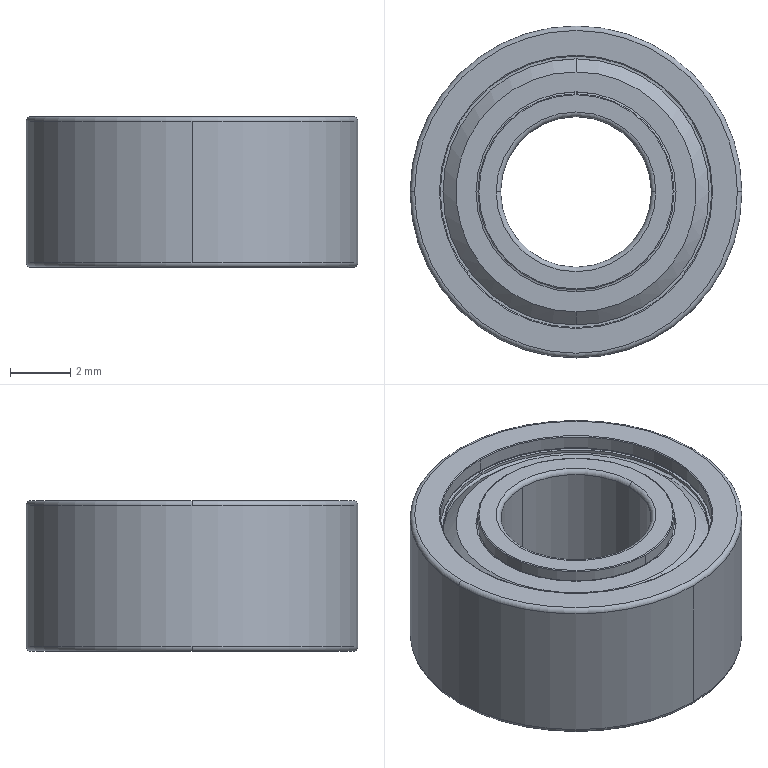Part | SolidWorks | features BaseBody 4 | 4 solids | 224 faces | box 11 x 11 x 5 mm | volume 259.376 mm3 | torus 84 | sphere 60 | cylinder 36 | plane 32 | cone 12 | commonest cylinder face diameters 9 x8 6.5 x4 6.632 x4 6.75 x4 7 x4 8.823 x4